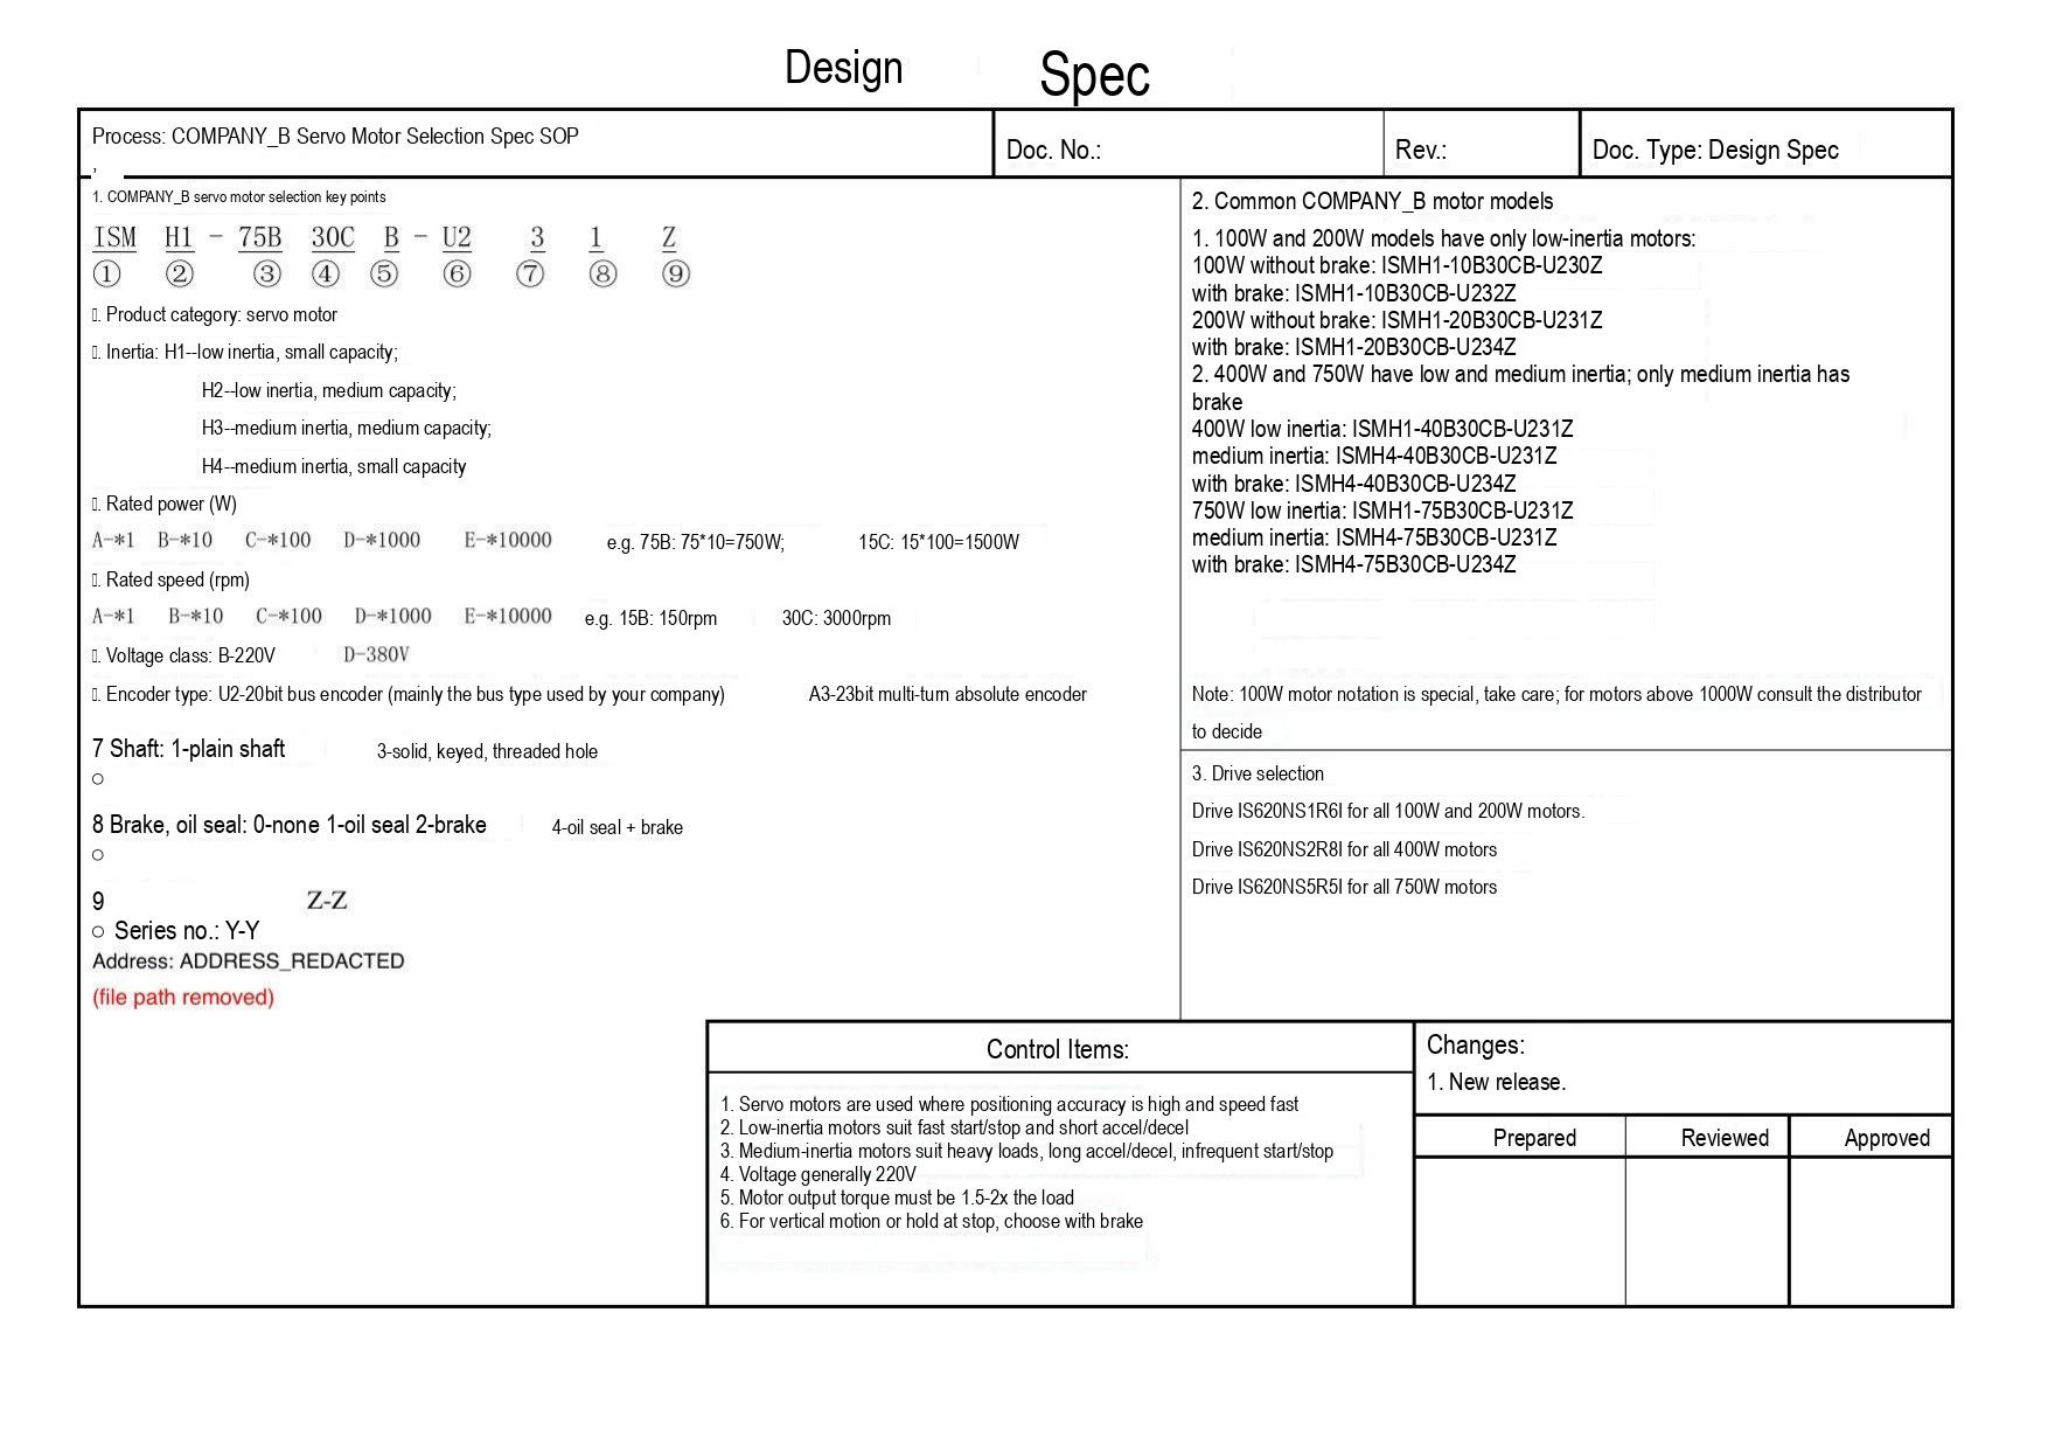Design Spec

| Process: COMPANY_B Servo Motor Selection Spec SOP | Doc. No.: | Rev.: | Doc. Type: Design Spec |
|---|---|---|---|

1. COMPANY_B servo motor selection key points

ISM H1 - 75B 30C B - U2 3 1 Z
① ② ③ ④ ⑤ ⑥ ⑦ ⑧ ⑨

Product category: servo motor

Inertia: H1--low inertia, small capacity;
H2--low inertia, medium capacity;
H3--medium inertia, medium capacity;
H4--medium inertia, small capacity

Rated power (W)
A-*1 B-*10 C-*100 D-*1000 E-*10000 e.g. 75B: 75*10=750W; 15C: 15*100=1500W

Rated speed (rpm)
A-*1 B-*10 C-*100 D-*1000 E-*10000 e.g. 15B: 150rpm 30C: 3000rpm

Voltage class: B-220V D-380V

Encoder type: U2-20bit bus encoder (mainly the bus type used by your company) A3-23bit multi-turn absolute encoder

7 Shaft: 1-plain shaft 3-solid, keyed, threaded hole
○

8 Brake, oil seal: 0-none 1-oil seal 2-brake 4-oil seal + brake
○

9 Z-Z
○ Series no.: Y-Y

Address: ADDRESS_REDACTED
(file path removed)

2. Common COMPANY_B motor models
1. 100W and 200W models have only low-inertia motors:
100W without brake: ISMH1-10B30CB-U230Z
with brake: ISMH1-10B30CB-U232Z
200W without brake: ISMH1-20B30CB-U231Z
with brake: ISMH1-20B30CB-U234Z
2. 400W and 750W have low and medium inertia; only medium inertia has brake
400W low inertia: ISMH1-40B30CB-U231Z
medium inertia: ISMH4-40B30CB-U231Z
with brake: ISMH4-40B30CB-U234Z
750W low inertia: ISMH1-75B30CB-U231Z
medium inertia: ISMH4-75B30CB-U231Z
with brake: ISMH4-75B30CB-U234Z

Note: 100W motor notation is special, take care; for motors above 1000W consult the distributor to decide

3. Drive selection
Drive IS620NS1R6I for all 100W and 200W motors.
Drive IS620NS2R8I for all 400W motors
Drive IS620NS5R5I for all 750W motors

Control Items:
1. Servo motors are used where positioning accuracy is high and speed fast
2. Low-inertia motors suit fast start/stop and short accel/decel
3. Medium-inertia motors suit heavy loads, long accel/decel, infrequent start/stop
4. Voltage generally 220V
5. Motor output torque must be 1.5-2x the load
6. For vertical motion or hold at stop, choose with brake

Changes:
1. New release.

| Prepared | Reviewed | Approved |
|---|---|---|
| | | |